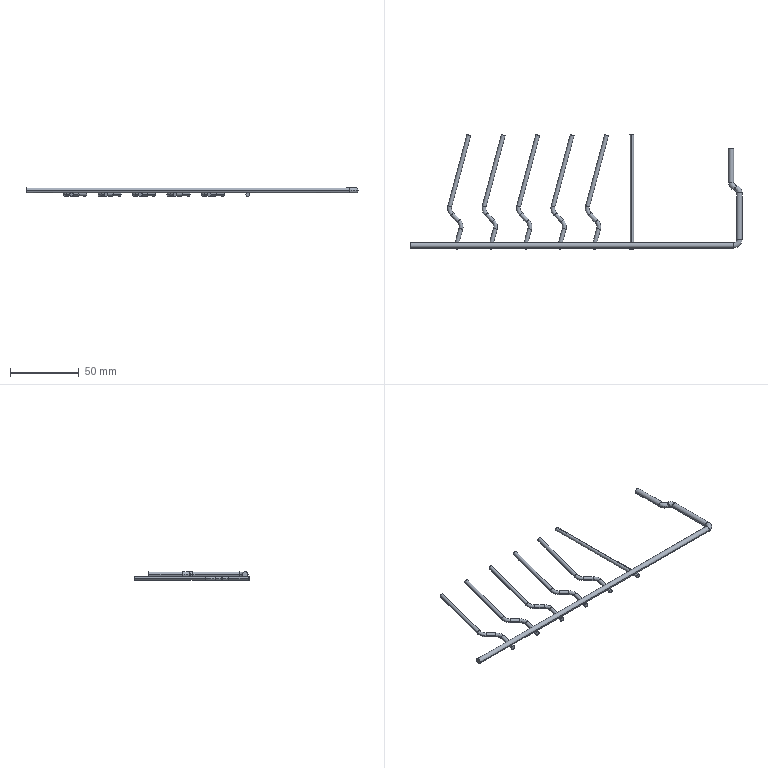Part | STEP file | ZXW722-L-178-B_21_1_1 | 1 solid | 80 faces | box 240.95 x 83.325 x 6.4 mm | volume 6922 mm3 | cylinder 40 | torus 26 | plane 14 | commonest cylinder face diameters 2.8 x32 3.9 x8